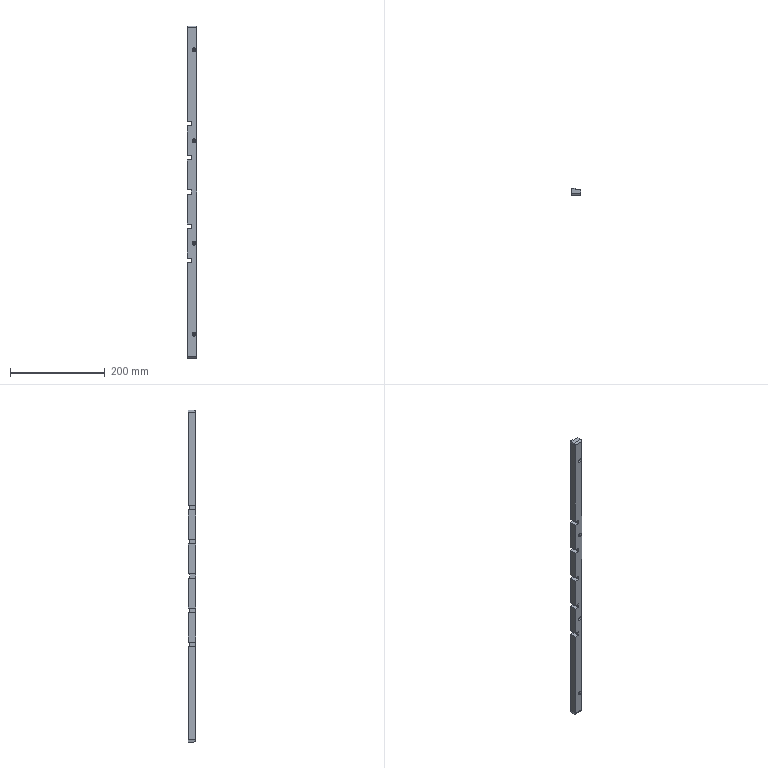Part | SolidWorks | features Chamfer 2, Extrusion 1, Fillet 1, HoleWzd 1, ICE 1 | 1 solid | 62 faces | box 20.5 x 15 x 700 mm | volume 182437 mm3 | plane 44 | cylinder 18 | commonest cylinder face diameters 8 x10 4.5 x8